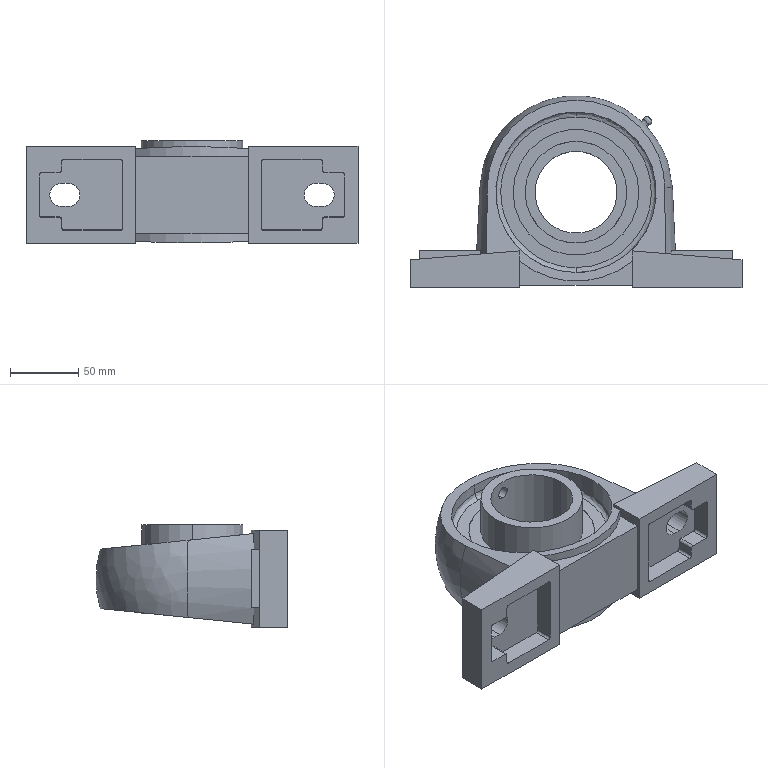Part | STEP file | 1 solid | 121 faces | box 243 x 140.56 x 75.2 mm | volume 669545 mm3 | plane 58 | cylinder 28 | spline 19 | cone 16 | commonest cylinder face diameters 74.5 x6 92.04 x6 117.457 x6 17 x4 8.918 x2 60 x2